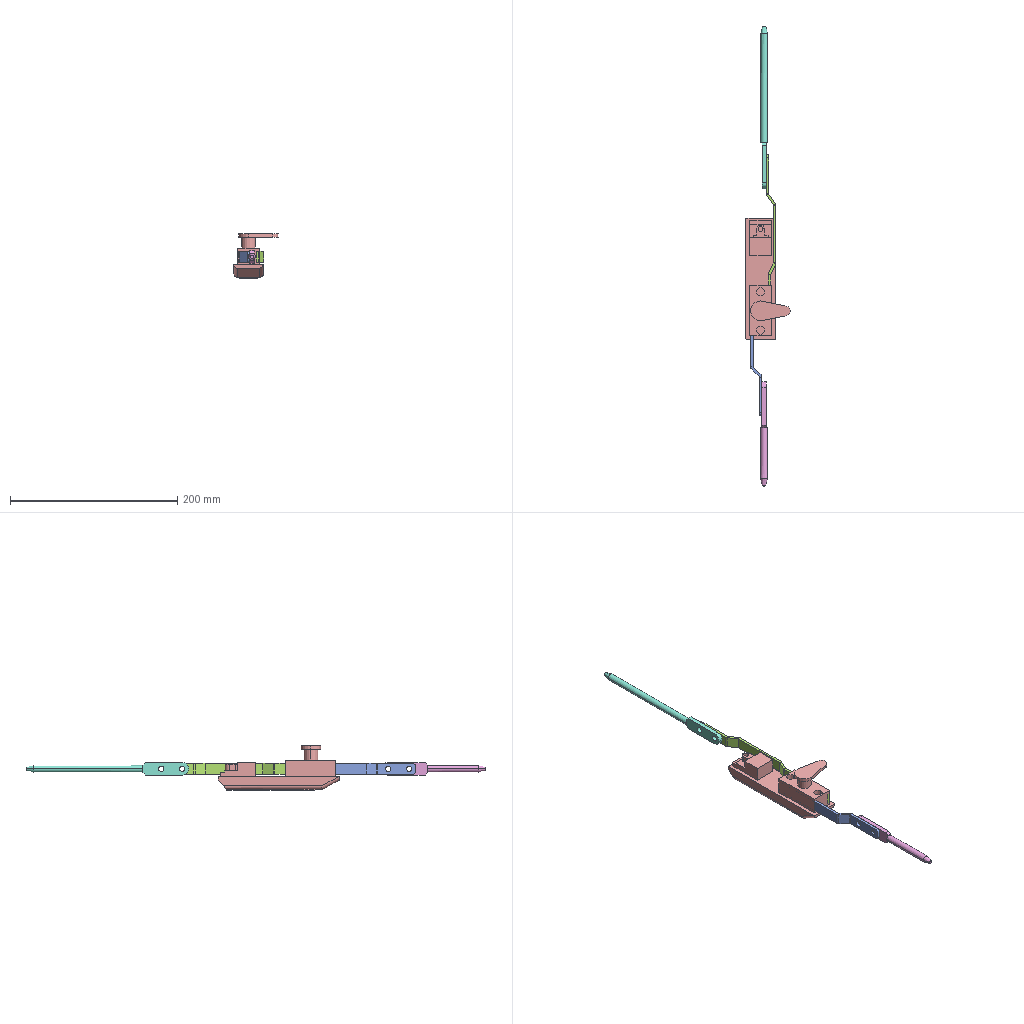Assembly | SolidWorks | 5 different items | 5 placed | box 53 x 551 x 53 mm
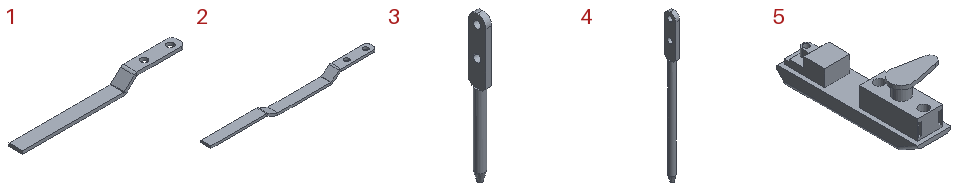Parts list (item | quantity | size | volume | features):
1 | x1 | 155.607 x 13 x 13.607 mm | 6013 mm3 | features EdgeFlange 2, Fillet 1, FlatPattern 1, ICE 1, SMBaseFlange 1, SheetMetal 1
2 | x1 | 216.882 x 13 x 11.604 mm | 8395 mm3 | features EdgeFlange 4, Fillet 1, FlatPattern 1, ICE 1, SMBaseFlange 1, SheetMetal 1
3 | x1 | 8 x 15 x 125 mm | 6966 mm3 | features ICE 2, Chamfer 1, Extrusion 1, Fillet 1, RevCut 1
4 | x1 | 8 x 15 x 195 mm | 10485 mm3 | features ICE 2, Chamfer 1, Extrusion 1, Fillet 1, RevCut 1
5 | x1 | 52.826 x 145 x 53 mm | 113904 mm3 | features ICE 19, CutThin 2, Fillet 2, Chamfer 1, Extrusion 1
Mates (type | each side: item.copy, entity, surface, feature):
Coincident | 5.1 face plane Cut-Extrude19 | 1.1 face plane Base-Flange1 | 2 times
Coincident | 5.1 face plane Cut-Extrude19 | 2.1 face plane Base-Flange1 | 2 times
Concentric | 1.1 face cylinder Cut-Extrude1 | 3.1 face cylinder Cut-Extrude4 | 2 times
Coincident | 1.1 face plane Edge-Flange2 | 3.1 face plane Boss-Extrude2
Concentric | 2.1 face cylinder Cut-Extrude1 | 4.1 face cylinder Cut-Extrude4 | 2 times
Coincident | 2.1 face plane Edge-Flange4 | 4.1 face plane Boss-Extrude2